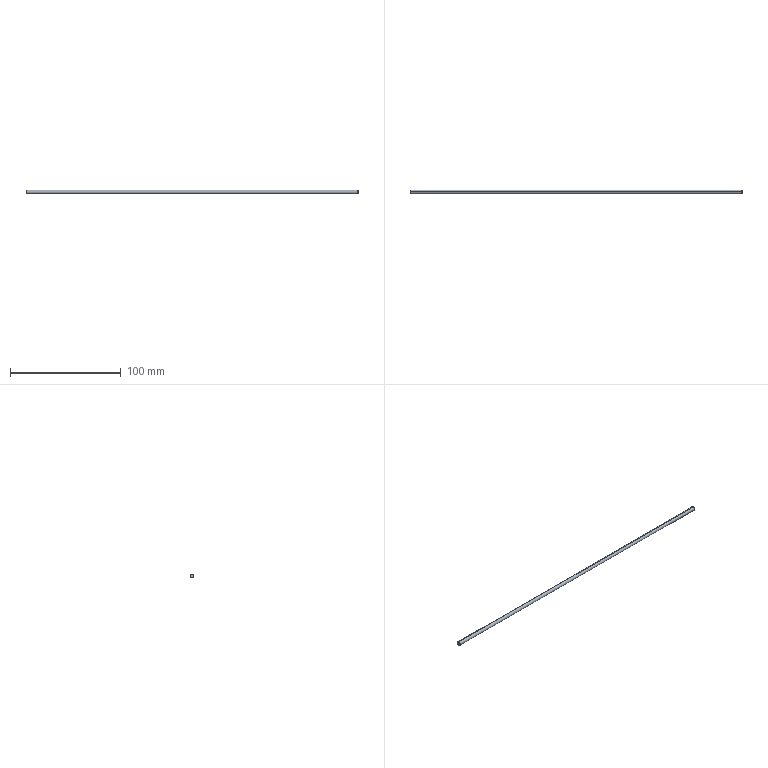Part | SolidWorks | features StudWizard 2, Extrusion 1 | 1 solid | 8 faces | box 300 x 3.5 x 3.5 mm | volume 2885 mm3 | cone 4 | cylinder 2 | plane 2 | commonest cylinder face diameters 3.5 x2
STEP:
#1=CARTESIAN_POINT('',(-300.,0.,-1.415));
#2=VERTEX_POINT('',#1);
#3=CARTESIAN_POINT('',(-300.,0.,1.415));
#4=VERTEX_POINT('',#3);
#5=CARTESIAN_POINT('',(-300.,0.,0.));
#6=DIRECTION('',(1.,0.,0.));
#7=DIRECTION('',(0.,0.,-1.));
#8=AXIS2_PLACEMENT_3D('',#5,#6,#7);
#9=CIRCLE('',#8,1.415);
#10=EDGE_CURVE('',#2,#4,#9,.T.);
#11=ORIENTED_EDGE('',*,*,#10,.T.);
#12=CARTESIAN_POINT('',(-299.664,0.,1.75));
#13=VERTEX_POINT('',#12);
#14=CARTESIAN_POINT('',(-300.,0.,1.415));
#15=DIRECTION('',(0.7071,0.,0.7071));
#16=VECTOR('',#15,1000.);
#17=LINE('',#14,#16);
#18=EDGE_CURVE('',#4,#13,#17,.T.);
#19=ORIENTED_EDGE('',*,*,#18,.T.);
#20=CARTESIAN_POINT('',(-299.664,0.,-1.75));
#21=VERTEX_POINT('',#20);
#22=CARTESIAN_POINT('',(-299.664,0.,0.));
#23=DIRECTION('',(1.,0.,0.));
#24=DIRECTION('',(0.,0.,-1.));
#25=AXIS2_PLACEMENT_3D('',#22,#23,#24);
#26=CIRCLE('',#25,1.75);
#27=EDGE_CURVE('',#21,#13,#26,.T.);
#28=ORIENTED_EDGE('',*,*,#27,.F.);
#29=CARTESIAN_POINT('',(-300.,0.,-1.415));
#30=DIRECTION('',(0.7071,0.,-0.7071));
#31=VECTOR('',#30,1000.);
#32=LINE('',#29,#31);
#33=EDGE_CURVE('',#2,#21,#32,.T.);
#34=ORIENTED_EDGE('',*,*,#33,.F.);
#35=EDGE_LOOP('',(#11,#19,#28,#34));
#36=FACE_OUTER_BOUND('',#35,.T.);
#37=CARTESIAN_POINT('',(-300.,0.,0.));
#38=DIRECTION('',(1.,0.,0.));
#39=DIRECTION('',(0.,0.,-1.));
#40=AXIS2_PLACEMENT_3D('',#37,#38,#39);
#41=CONICAL_SURFACE('',#40,1.415,0.7854);
#42=ADVANCED_FACE('',(#36),#41,.T.);
#43=CARTESIAN_POINT('',(0.,0.,1.415));
#44=VERTEX_POINT('',#43);
#45=CARTESIAN_POINT('',(0.,0.,-1.415));
#46=VERTEX_POINT('',#45);
#47=CARTESIAN_POINT('',(0.,0.,0.));
#48=DIRECTION('',(-1.,0.,0.));
#49=DIRECTION('',(0.,0.,1.));
#50=AXIS2_PLACEMENT_3D('',#47,#48,#49);
#51=CIRCLE('',#50,1.415);
#52=EDGE_CURVE('',#44,#46,#51,.T.);
#53=ORIENTED_EDGE('',*,*,#52,.T.);
#54=CARTESIAN_POINT('',(-0.3355,0.,-1.75));
#55=VERTEX_POINT('',#54);
#56=CARTESIAN_POINT('',(0.,0.,-1.415));
#57=DIRECTION('',(-0.7071,0.,-0.7071));
#58=VECTOR('',#57,1000.);
#59=LINE('',#56,#58);
#60=EDGE_CURVE('',#46,#55,#59,.T.);
#61=ORIENTED_EDGE('',*,*,#60,.T.);
#62=CARTESIAN_POINT('',(-0.3355,0.,1.75));
#63=VERTEX_POINT('',#62);
#64=CARTESIAN_POINT('',(-0.3355,0.,0.));
#65=DIRECTION('',(-1.,0.,0.));
#66=DIRECTION('',(0.,0.,1.));
#67=AXIS2_PLACEMENT_3D('',#64,#65,#66);
#68=CIRCLE('',#67,1.75);
#69=EDGE_CURVE('',#63,#55,#68,.T.);
#70=ORIENTED_EDGE('',*,*,#69,.F.);
#71=CARTESIAN_POINT('',(0.,0.,1.415));
#72=DIRECTION('',(-0.7071,0.,0.7071));
#73=VECTOR('',#72,1000.);
#74=LINE('',#71,#73);
#75=EDGE_CURVE('',#44,#63,#74,.T.);
#76=ORIENTED_EDGE('',*,*,#75,.F.);
#77=EDGE_LOOP('',(#53,#61,#70,#76));
#78=FACE_OUTER_BOUND('',#77,.T.);
#79=CARTESIAN_POINT('',(0.,0.,0.));
#80=DIRECTION('',(-1.,0.,0.));
#81=DIRECTION('',(0.,0.,1.));
#82=AXIS2_PLACEMENT_3D('',#79,#80,#81);
#83=CONICAL_SURFACE('',#82,1.415,0.7854);
#84=ADVANCED_FACE('',(#78),#83,.T.);
#85=ORIENTED_EDGE('',*,*,#27,.T.);
#86=CARTESIAN_POINT('',(-300.,0.,1.75));
#87=DIRECTION('',(1.,0.,0.));
#88=VECTOR('',#87,1000.);
#89=LINE('',#86,#88);
#90=EDGE_CURVE('',#13,#63,#89,.T.);
#91=ORIENTED_EDGE('',*,*,#90,.T.);
#92=ORIENTED_EDGE('',*,*,#69,.T.);
#93=CARTESIAN_POINT('',(-300.,0.,-1.75));
#94=DIRECTION('',(1.,0.,0.));
#95=VECTOR('',#94,1000.);
#96=LINE('',#93,#95);
#97=EDGE_CURVE('',#21,#55,#96,.T.);
#98=ORIENTED_EDGE('',*,*,#97,.F.);
#99=EDGE_LOOP('',(#85,#91,#92,#98));
#100=FACE_OUTER_BOUND('',#99,.T.);
#101=CARTESIAN_POINT('',(-300.,0.,0.));
#102=DIRECTION('',(1.,0.,0.));
#103=DIRECTION('',(0.,0.,-1.));
#104=AXIS2_PLACEMENT_3D('',#101,#102,#103);
#105=CYLINDRICAL_SURFACE('',#104,1.75);
#106=ADVANCED_FACE('',(#100),#105,.T.);
#107=ORIENTED_EDGE('',*,*,#90,.F.);
#108=CARTESIAN_POINT('',(-299.664,0.,0.));
#109=DIRECTION('',(1.,0.,0.));
#110=DIRECTION('',(0.,0.,-1.));
#111=AXIS2_PLACEMENT_3D('',#108,#109,#110);
#112=CIRCLE('',#111,1.75);
#113=EDGE_CURVE('',#13,#21,#112,.T.);
#114=ORIENTED_EDGE('',*,*,#113,.T.);
#115=ORIENTED_EDGE('',*,*,#97,.T.);
#116=CARTESIAN_POINT('',(-0.3355,0.,0.));
#117=DIRECTION('',(-1.,0.,0.));
#118=DIRECTION('',(0.,0.,1.));
#119=AXIS2_PLACEMENT_3D('',#116,#117,#118);
#120=CIRCLE('',#119,1.75);
#121=EDGE_CURVE('',#55,#63,#120,.T.);
#122=ORIENTED_EDGE('',*,*,#121,.T.);
#123=EDGE_LOOP('',(#107,#114,#115,#122));
#124=FACE_OUTER_BOUND('',#123,.T.);
#125=CARTESIAN_POINT('',(-300.,0.,0.));
#126=DIRECTION('',(1.,0.,0.));
#127=DIRECTION('',(0.,0.,-1.));
#128=AXIS2_PLACEMENT_3D('',#125,#126,#127);
#129=CYLINDRICAL_SURFACE('',#128,1.75);
#130=ADVANCED_FACE('',(#124),#129,.T.);
#131=ORIENTED_EDGE('',*,*,#60,.F.);
#132=CARTESIAN_POINT('',(0.,0.,0.));
#133=DIRECTION('',(-1.,0.,0.));
#134=DIRECTION('',(0.,0.,1.));
#135=AXIS2_PLACEMENT_3D('',#132,#133,#134);
#136=CIRCLE('',#135,1.415);
#137=EDGE_CURVE('',#46,#44,#136,.T.);
#138=ORIENTED_EDGE('',*,*,#137,.T.);
#139=ORIENTED_EDGE('',*,*,#75,.T.);
#140=ORIENTED_EDGE('',*,*,#121,.F.);
#141=EDGE_LOOP('',(#131,#138,#139,#140));
#142=FACE_OUTER_BOUND('',#141,.T.);
#143=CARTESIAN_POINT('',(0.,0.,0.));
#144=DIRECTION('',(-1.,0.,0.));
#145=DIRECTION('',(0.,0.,1.));
#146=AXIS2_PLACEMENT_3D('',#143,#144,#145);
#147=CONICAL_SURFACE('',#146,1.415,0.7854);
#148=ADVANCED_FACE('',(#142),#147,.T.);
#149=ORIENTED_EDGE('',*,*,#52,.F.);
#150=ORIENTED_EDGE('',*,*,#137,.F.);
#151=EDGE_LOOP('',(#149,#150));
#152=FACE_OUTER_BOUND('',#151,.T.);
#153=CARTESIAN_POINT('',(0.,0.,0.));
#154=DIRECTION('',(1.,0.,0.));
#155=DIRECTION('',(0.,0.,-1.));
#156=AXIS2_PLACEMENT_3D('',#153,#154,#155);
#157=PLANE('',#156);
#158=ADVANCED_FACE('',(#152),#157,.T.);
#159=ORIENTED_EDGE('',*,*,#18,.F.);
#160=CARTESIAN_POINT('',(-300.,0.,0.));
#161=DIRECTION('',(1.,0.,0.));
#162=DIRECTION('',(0.,0.,-1.));
#163=AXIS2_PLACEMENT_3D('',#160,#161,#162);
#164=CIRCLE('',#163,1.415);
#165=EDGE_CURVE('',#4,#2,#164,.T.);
#166=ORIENTED_EDGE('',*,*,#165,.T.);
#167=ORIENTED_EDGE('',*,*,#33,.T.);
#168=ORIENTED_EDGE('',*,*,#113,.F.);
#169=EDGE_LOOP('',(#159,#166,#167,#168));
#170=FACE_OUTER_BOUND('',#169,.T.);
#171=CARTESIAN_POINT('',(-300.,0.,0.));
#172=DIRECTION('',(1.,0.,0.));
#173=DIRECTION('',(0.,0.,-1.));
#174=AXIS2_PLACEMENT_3D('',#171,#172,#173);
#175=CONICAL_SURFACE('',#174,1.415,0.7854);
#176=ADVANCED_FACE('',(#170),#175,.T.);
#177=ORIENTED_EDGE('',*,*,#10,.F.);
#178=ORIENTED_EDGE('',*,*,#165,.F.);
#179=EDGE_LOOP('',(#177,#178));
#180=FACE_OUTER_BOUND('',#179,.T.);
#181=CARTESIAN_POINT('',(-300.,0.,0.));
#182=DIRECTION('',(1.,0.,0.));
#183=DIRECTION('',(0.,0.,-1.));
#184=AXIS2_PLACEMENT_3D('',#181,#182,#183);
#185=PLANE('',#184);
#186=ADVANCED_FACE('',(#180),#185,.F.);
#187=CLOSED_SHELL('',(#42,#84,#106,#130,#148,#158,#176,#186));
#188=MANIFOLD_SOLID_BREP('',#187);
#189=CARTESIAN_POINT('',(0.,0.,0.));
#190=DIRECTION('',(0.,0.,1.));
#191=DIRECTION('',(1.,0.,0.));
#192=AXIS2_PLACEMENT_3D('',#189,#190,#191);
#193=(LENGTH_UNIT()NAMED_UNIT(*)SI_UNIT(.MILLI.,.METRE.));
#194=UNCERTAINTY_MEASURE_WITH_UNIT(LENGTH_MEASURE(0.00001),#193,'','');
#195=(NAMED_UNIT(*)PLANE_ANGLE_UNIT()SI_UNIT($,.RADIAN.));
#196=(NAMED_UNIT(*)SI_UNIT($,.STERADIAN.)SOLID_ANGLE_UNIT());
#197=(GEOMETRIC_REPRESENTATION_CONTEXT(3)GLOBAL_UNCERTAINTY_ASSIGNED_CONTEXT((#194))GLOBAL_UNIT_ASSIGNED_CONTEXT((#193,#195,#196))REPRESENTATION_CONTEXT('',''));
#198=ADVANCED_BREP_SHAPE_REPRESENTATION('',(#188,#192),#197);